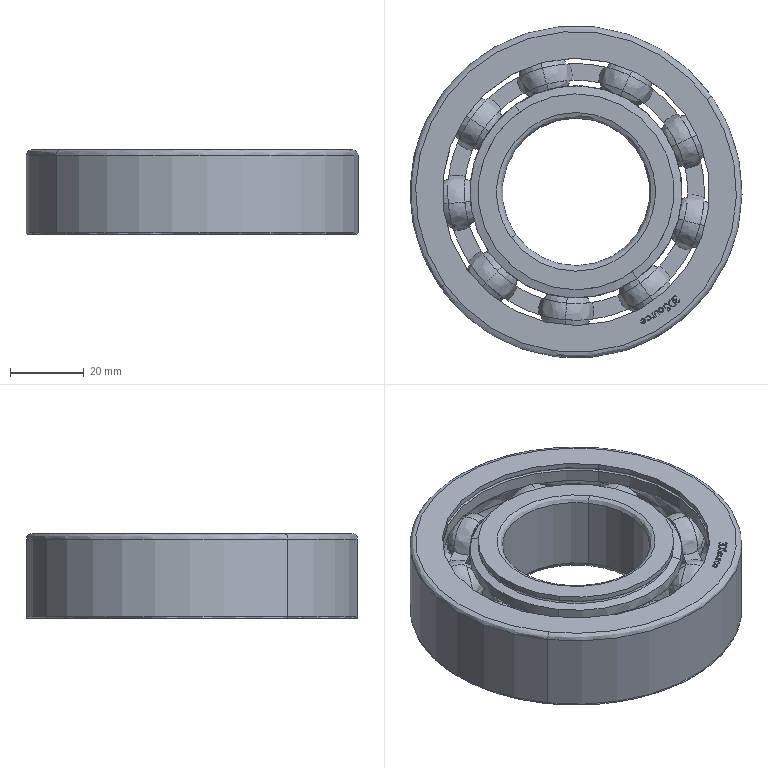Part | SolidWorks | features BaseBody 14 | 12 solids | 225 faces | box 90 x 90 x 23 mm | volume 82930 mm3 | spline 98 | plane 66 | cylinder 57 | cone 4 | commonest cylinder face diameters 72.5 x8 0.806 x7 1.401 x6 0.999 x5 1.2 x4 53.125 x4